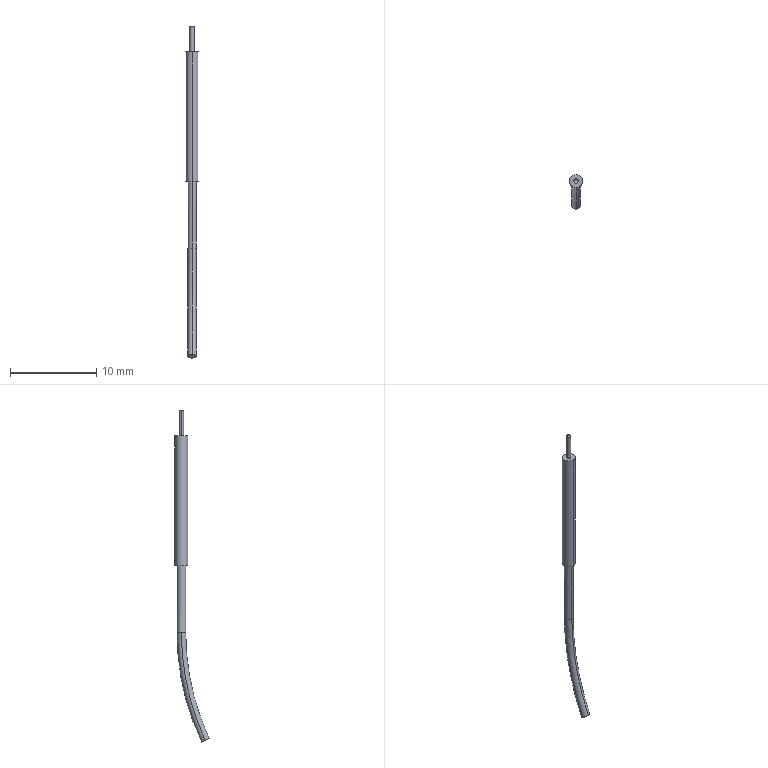Part | NX | 1 solid | 16 faces | box 1.5 x 3.958 x 38.402 mm | volume 43.25 mm3 | cylinder 8 | plane 5 | torus 3 | commonest cylinder face diameters 0.49 x2 0.5 x2 1 x2 1.5 x2
STEP:
#1=CARTESIAN_POINT('',(0.25,0.,3.));
#2=VERTEX_POINT('',#1);
#3=CARTESIAN_POINT('',(-0.25,0.,3.));
#4=VERTEX_POINT('',#3);
#5=CARTESIAN_POINT('',(0.,0.,3.));
#6=DIRECTION('',(0.,0.,-1.));
#7=DIRECTION('',(1.,0.,0.));
#8=AXIS2_PLACEMENT_3D('',#5,#6,#7);
#9=CIRCLE('',#8,0.25);
#10=EDGE_CURVE('',#2,#4,#9,.T.);
#11=ORIENTED_EDGE('',*,*,#10,.F.);
#12=CARTESIAN_POINT('',(0.,0.,3.));
#13=DIRECTION('',(0.,0.,-1.));
#14=DIRECTION('',(1.,0.,0.));
#15=AXIS2_PLACEMENT_3D('',#12,#13,#14);
#16=CIRCLE('',#15,0.25);
#17=EDGE_CURVE('',#4,#2,#16,.T.);
#18=ORIENTED_EDGE('',*,*,#17,.F.);
#19=EDGE_LOOP('',(#11,#18));
#20=FACE_BOUND('',#19,.T.);
#21=CARTESIAN_POINT('',(-0.245,0.,3.));
#22=VERTEX_POINT('',#21);
#23=CARTESIAN_POINT('',(0.245,0.,3.));
#24=VERTEX_POINT('',#23);
#25=CARTESIAN_POINT('',(0.,0.,3.));
#26=DIRECTION('',(0.,0.,1.));
#27=DIRECTION('',(1.,0.,0.));
#28=AXIS2_PLACEMENT_3D('',#25,#26,#27);
#29=CIRCLE('',#28,0.245);
#30=EDGE_CURVE('',#22,#24,#29,.T.);
#31=ORIENTED_EDGE('',*,*,#30,.F.);
#32=CARTESIAN_POINT('',(0.,0.,3.));
#33=DIRECTION('',(0.,0.,1.));
#34=DIRECTION('',(1.,0.,0.));
#35=AXIS2_PLACEMENT_3D('',#32,#33,#34);
#36=CIRCLE('',#35,0.245);
#37=EDGE_CURVE('',#24,#22,#36,.T.);
#38=ORIENTED_EDGE('',*,*,#37,.F.);
#39=EDGE_LOOP('',(#31,#38));
#40=FACE_BOUND('',#39,.T.);
#41=CARTESIAN_POINT('',(0.,0.,3.));
#42=DIRECTION('',(0.,0.,1.));
#43=DIRECTION('',(1.,0.,0.));
#44=AXIS2_PLACEMENT_3D('',#41,#42,#43);
#45=PLANE('',#44);
#46=ADVANCED_FACE('',(#20,#40),#45,.T.);
#47=ORIENTED_EDGE('',*,*,#10,.T.);
#48=CARTESIAN_POINT('',(-0.25,0.,0.));
#49=VERTEX_POINT('',#48);
#50=CARTESIAN_POINT('',(-0.25,0.,0.));
#51=DIRECTION('',(0.,0.,1.));
#52=VECTOR('',#51,1000.);
#53=LINE('',#50,#52);
#54=EDGE_CURVE('',#49,#4,#53,.T.);
#55=ORIENTED_EDGE('',*,*,#54,.F.);
#56=CARTESIAN_POINT('',(0.25,0.,0.));
#57=VERTEX_POINT('',#56);
#58=CARTESIAN_POINT('',(0.,0.,0.));
#59=DIRECTION('',(0.,0.,1.));
#60=DIRECTION('',(-1.,0.,0.));
#61=AXIS2_PLACEMENT_3D('',#58,#59,#60);
#62=CIRCLE('',#61,0.25);
#63=EDGE_CURVE('',#49,#57,#62,.T.);
#64=ORIENTED_EDGE('',*,*,#63,.T.);
#65=CARTESIAN_POINT('',(0.25,0.,0.));
#66=DIRECTION('',(0.,0.,1.));
#67=VECTOR('',#66,1000.);
#68=LINE('',#65,#67);
#69=EDGE_CURVE('',#57,#2,#68,.T.);
#70=ORIENTED_EDGE('',*,*,#69,.T.);
#71=EDGE_LOOP('',(#47,#55,#64,#70));
#72=FACE_BOUND('',#71,.T.);
#73=CARTESIAN_POINT('',(0.,0.,0.));
#74=DIRECTION('',(0.,0.,1.));
#75=DIRECTION('',(1.,0.,0.));
#76=AXIS2_PLACEMENT_3D('',#73,#74,#75);
#77=CYLINDRICAL_SURFACE('',#76,0.25);
#78=ADVANCED_FACE('',(#72),#77,.T.);
#79=CARTESIAN_POINT('',(0.,-0.75,0.));
#80=VERTEX_POINT('',#79);
#81=CARTESIAN_POINT('',(0.,0.75,0.));
#82=VERTEX_POINT('',#81);
#83=CARTESIAN_POINT('',(0.,0.,0.));
#84=DIRECTION('',(0.,0.,-1.));
#85=DIRECTION('',(0.,1.,0.));
#86=AXIS2_PLACEMENT_3D('',#83,#84,#85);
#87=CIRCLE('',#86,0.75);
#88=EDGE_CURVE('',#80,#82,#87,.T.);
#89=ORIENTED_EDGE('',*,*,#88,.F.);
#90=CARTESIAN_POINT('',(0.,0.,0.));
#91=DIRECTION('',(0.,0.,-1.));
#92=DIRECTION('',(0.,1.,0.));
#93=AXIS2_PLACEMENT_3D('',#90,#91,#92);
#94=CIRCLE('',#93,0.75);
#95=EDGE_CURVE('',#82,#80,#94,.T.);
#96=ORIENTED_EDGE('',*,*,#95,.F.);
#97=EDGE_LOOP('',(#89,#96));
#98=FACE_BOUND('',#97,.T.);
#99=ORIENTED_EDGE('',*,*,#63,.F.);
#100=CARTESIAN_POINT('',(0.,0.,0.));
#101=DIRECTION('',(0.,0.,1.));
#102=DIRECTION('',(-1.,0.,0.));
#103=AXIS2_PLACEMENT_3D('',#100,#101,#102);
#104=CIRCLE('',#103,0.25);
#105=EDGE_CURVE('',#57,#49,#104,.T.);
#106=ORIENTED_EDGE('',*,*,#105,.F.);
#107=EDGE_LOOP('',(#99,#106));
#108=FACE_BOUND('',#107,.T.);
#109=CARTESIAN_POINT('',(0.,0.,0.));
#110=DIRECTION('',(0.,0.,-1.));
#111=DIRECTION('',(0.,-1.,0.));
#112=AXIS2_PLACEMENT_3D('',#109,#110,#111);
#113=PLANE('',#112);
#114=ADVANCED_FACE('',(#98,#108),#113,.F.);
#115=CARTESIAN_POINT('',(0.,0.75,-15.));
#116=VERTEX_POINT('',#115);
#117=CARTESIAN_POINT('',(0.,-0.75,-15.));
#118=VERTEX_POINT('',#117);
#119=CARTESIAN_POINT('',(0.,0.,-15.));
#120=DIRECTION('',(0.,0.,1.));
#121=DIRECTION('',(0.,1.,0.));
#122=AXIS2_PLACEMENT_3D('',#119,#120,#121);
#123=CIRCLE('',#122,0.75);
#124=EDGE_CURVE('',#116,#118,#123,.T.);
#125=ORIENTED_EDGE('',*,*,#124,.T.);
#126=CARTESIAN_POINT('',(0.,-0.75,0.));
#127=DIRECTION('',(0.,0.,-1.));
#128=VECTOR('',#127,1000.);
#129=LINE('',#126,#128);
#130=EDGE_CURVE('',#118,#80,#129,.F.);
#131=ORIENTED_EDGE('',*,*,#130,.T.);
#132=ORIENTED_EDGE('',*,*,#88,.T.);
#133=CARTESIAN_POINT('',(0.,0.75,0.));
#134=DIRECTION('',(0.,0.,-1.));
#135=VECTOR('',#134,1000.);
#136=LINE('',#133,#135);
#137=EDGE_CURVE('',#116,#82,#136,.F.);
#138=ORIENTED_EDGE('',*,*,#137,.F.);
#139=EDGE_LOOP('',(#125,#131,#132,#138));
#140=FACE_BOUND('',#139,.T.);
#141=CARTESIAN_POINT('',(0.,0.,0.));
#142=DIRECTION('',(0.,0.,-1.));
#143=DIRECTION('',(0.,-1.,0.));
#144=AXIS2_PLACEMENT_3D('',#141,#142,#143);
#145=CYLINDRICAL_SURFACE('',#144,0.75);
#146=ADVANCED_FACE('',(#140),#145,.T.);
#147=CARTESIAN_POINT('',(-0.5,-2.754,-35.192));
#148=VERTEX_POINT('',#147);
#149=CARTESIAN_POINT('',(0.,-3.208,-34.982));
#150=VERTEX_POINT('',#149);
#151=CARTESIAN_POINT('',(0.,-2.754,-35.192));
#152=DIRECTION('',(0.,0.4199,0.9076));
#153=DIRECTION('',(0.,-0.9076,0.4199));
#154=AXIS2_PLACEMENT_3D('',#151,#152,#153);
#155=CIRCLE('',#154,0.5);
#156=EDGE_CURVE('',#148,#150,#155,.T.);
#157=ORIENTED_EDGE('',*,*,#156,.F.);
#158=CARTESIAN_POINT('',(0.5,-2.754,-35.192));
#159=VERTEX_POINT('',#158);
#160=CARTESIAN_POINT('',(0.,-2.754,-35.192));
#161=DIRECTION('',(0.,0.4199,0.9076));
#162=DIRECTION('',(0.,-0.9076,0.4199));
#163=AXIS2_PLACEMENT_3D('',#160,#161,#162);
#164=CIRCLE('',#163,0.5);
#165=EDGE_CURVE('',#159,#148,#164,.T.);
#166=ORIENTED_EDGE('',*,*,#165,.F.);
#167=CARTESIAN_POINT('',(0.,-2.754,-35.192));
#168=DIRECTION('',(0.,0.4199,0.9076));
#169=DIRECTION('',(0.,-0.9076,0.4199));
#170=AXIS2_PLACEMENT_3D('',#167,#168,#169);
#171=CIRCLE('',#170,0.5);
#172=EDGE_CURVE('',#150,#159,#171,.T.);
#173=ORIENTED_EDGE('',*,*,#172,.F.);
#174=EDGE_LOOP('',(#157,#166,#173));
#175=FACE_BOUND('',#174,.T.);
#176=CARTESIAN_POINT('',(1.,-29.794,-22.681));
#177=DIRECTION('',(0.,-0.4199,-0.9076));
#178=DIRECTION('',(0.,-0.9076,0.4199));
#179=AXIS2_PLACEMENT_3D('',#176,#177,#178);
#180=PLANE('',#179);
#181=ADVANCED_FACE('',(#175),#180,.T.);
#182=ORIENTED_EDGE('',*,*,#124,.F.);
#183=CARTESIAN_POINT('',(0.,0.,-15.));
#184=DIRECTION('',(0.,0.,1.));
#185=DIRECTION('',(0.,1.,0.));
#186=AXIS2_PLACEMENT_3D('',#183,#184,#185);
#187=CIRCLE('',#186,0.75);
#188=EDGE_CURVE('',#118,#116,#187,.T.);
#189=ORIENTED_EDGE('',*,*,#188,.F.);
#190=EDGE_LOOP('',(#182,#189));
#191=FACE_BOUND('',#190,.T.);
#192=CARTESIAN_POINT('',(0.,0.5,-15.));
#193=VERTEX_POINT('',#192);
#194=CARTESIAN_POINT('',(0.,-0.5,-15.));
#195=VERTEX_POINT('',#194);
#196=CARTESIAN_POINT('',(0.,0.,-15.));
#197=DIRECTION('',(0.,0.,-1.));
#198=DIRECTION('',(0.,-1.,0.));
#199=AXIS2_PLACEMENT_3D('',#196,#197,#198);
#200=CIRCLE('',#199,0.5);
#201=EDGE_CURVE('',#193,#195,#200,.T.);
#202=ORIENTED_EDGE('',*,*,#201,.F.);
#203=CARTESIAN_POINT('',(0.,0.,-15.));
#204=DIRECTION('',(0.,0.,-1.));
#205=DIRECTION('',(0.,-1.,0.));
#206=AXIS2_PLACEMENT_3D('',#203,#204,#205);
#207=CIRCLE('',#206,0.5);
#208=EDGE_CURVE('',#195,#193,#207,.T.);
#209=ORIENTED_EDGE('',*,*,#208,.F.);
#210=EDGE_LOOP('',(#202,#209));
#211=FACE_BOUND('',#210,.T.);
#212=CARTESIAN_POINT('',(0.,0.,-15.));
#213=DIRECTION('',(0.,0.,-1.));
#214=DIRECTION('',(0.,-1.,0.));
#215=AXIS2_PLACEMENT_3D('',#212,#213,#214);
#216=PLANE('',#215);
#217=ADVANCED_FACE('',(#191,#211),#216,.T.);
#218=ORIENTED_EDGE('',*,*,#201,.T.);
#219=CARTESIAN_POINT('',(0.,-0.5,-22.681));
#220=VERTEX_POINT('',#219);
#221=CARTESIAN_POINT('',(0.,-0.5,-15.));
#222=DIRECTION('',(0.,0.,-1.));
#223=VECTOR('',#222,1000.);
#224=LINE('',#221,#223);
#225=EDGE_CURVE('',#195,#220,#224,.T.);
#226=ORIENTED_EDGE('',*,*,#225,.T.);
#227=CARTESIAN_POINT('',(0.5,0.,-22.681));
#228=VERTEX_POINT('',#227);
#229=CARTESIAN_POINT('',(0.,0.,-22.681));
#230=DIRECTION('',(0.,0.,-1.));
#231=DIRECTION('',(-1.,0.,0.));
#232=AXIS2_PLACEMENT_3D('',#229,#230,#231);
#233=CIRCLE('',#232,0.5);
#234=EDGE_CURVE('',#228,#220,#233,.T.);
#235=ORIENTED_EDGE('',*,*,#234,.F.);
#236=CARTESIAN_POINT('',(0.,0.5,-22.681));
#237=VERTEX_POINT('',#236);
#238=CARTESIAN_POINT('',(0.,0.,-22.681));
#239=DIRECTION('',(0.,0.,-1.));
#240=DIRECTION('',(-1.,0.,0.));
#241=AXIS2_PLACEMENT_3D('',#238,#239,#240);
#242=CIRCLE('',#241,0.5);
#243=EDGE_CURVE('',#237,#228,#242,.T.);
#244=ORIENTED_EDGE('',*,*,#243,.F.);
#245=CARTESIAN_POINT('',(0.,0.5,-15.));
#246=DIRECTION('',(0.,0.,-1.));
#247=VECTOR('',#246,1000.);
#248=LINE('',#245,#247);
#249=EDGE_CURVE('',#193,#237,#248,.T.);
#250=ORIENTED_EDGE('',*,*,#249,.F.);
#251=EDGE_LOOP('',(#218,#226,#235,#244,#250));
#252=FACE_BOUND('',#251,.T.);
#253=CARTESIAN_POINT('',(0.,0.,-15.));
#254=DIRECTION('',(0.,0.,-1.));
#255=DIRECTION('',(0.,1.,0.));
#256=AXIS2_PLACEMENT_3D('',#253,#254,#255);
#257=CYLINDRICAL_SURFACE('',#256,0.5);
#258=ADVANCED_FACE('',(#252),#257,.T.);
#259=CARTESIAN_POINT('',(-0.245,0.,2.9));
#260=VERTEX_POINT('',#259);
#261=CARTESIAN_POINT('',(0.245,0.,2.9));
#262=VERTEX_POINT('',#261);
#263=CARTESIAN_POINT('',(0.,0.,2.9));
#264=DIRECTION('',(0.,0.,-1.));
#265=DIRECTION('',(-1.,0.,0.));
#266=AXIS2_PLACEMENT_3D('',#263,#264,#265);
#267=CIRCLE('',#266,0.245);
#268=EDGE_CURVE('',#260,#262,#267,.T.);
#269=ORIENTED_EDGE('',*,*,#268,.F.);
#270=CARTESIAN_POINT('',(0.,0.,2.9));
#271=DIRECTION('',(0.,0.,-1.));
#272=DIRECTION('',(-1.,0.,0.));
#273=AXIS2_PLACEMENT_3D('',#270,#271,#272);
#274=CIRCLE('',#273,0.245);
#275=EDGE_CURVE('',#262,#260,#274,.T.);
#276=ORIENTED_EDGE('',*,*,#275,.F.);
#277=EDGE_LOOP('',(#269,#276));
#278=FACE_BOUND('',#277,.T.);
#279=CARTESIAN_POINT('',(0.,0.,2.9));
#280=DIRECTION('',(0.,0.,1.));
#281=DIRECTION('',(1.,0.,0.));
#282=AXIS2_PLACEMENT_3D('',#279,#280,#281);
#283=PLANE('',#282);
#284=ADVANCED_FACE('',(#278),#283,.T.);
#285=CARTESIAN_POINT('',(0.,-29.794,-22.681));
#286=DIRECTION('',(-1.,0.,0.));
#287=DIRECTION('',(0.,0.,1.));
#288=AXIS2_PLACEMENT_3D('',#285,#286,#287);
#289=CIRCLE('',#288,29.294);
#290=EDGE_CURVE('',#220,#150,#289,.T.);
#291=ORIENTED_EDGE('',*,*,#290,.F.);
#292=CARTESIAN_POINT('',(-0.5,0.,-22.681));
#293=VERTEX_POINT('',#292);
#294=CARTESIAN_POINT('',(0.,0.,-22.681));
#295=DIRECTION('',(0.,0.,-1.));
#296=DIRECTION('',(-1.,0.,0.));
#297=AXIS2_PLACEMENT_3D('',#294,#295,#296);
#298=CIRCLE('',#297,0.5);
#299=EDGE_CURVE('',#220,#293,#298,.T.);
#300=ORIENTED_EDGE('',*,*,#299,.T.);
#301=CARTESIAN_POINT('',(-0.5,-29.794,-22.681));
#302=DIRECTION('',(-1.,0.,0.));
#303=DIRECTION('',(0.,1.,0.));
#304=AXIS2_PLACEMENT_3D('',#301,#302,#303);
#305=CIRCLE('',#304,29.794);
#306=EDGE_CURVE('',#293,#148,#305,.T.);
#307=ORIENTED_EDGE('',*,*,#306,.T.);
#308=ORIENTED_EDGE('',*,*,#156,.T.);
#309=EDGE_LOOP('',(#291,#300,#307,#308));
#310=FACE_BOUND('',#309,.T.);
#311=CARTESIAN_POINT('',(0.,-29.794,-22.681));
#312=DIRECTION('',(-1.,0.,0.));
#313=DIRECTION('',(0.,1.,0.));
#314=AXIS2_PLACEMENT_3D('',#311,#312,#313);
#315=TOROIDAL_SURFACE('',#314,29.794,0.5);
#316=ADVANCED_FACE('',(#310),#315,.T.);
#317=ORIENTED_EDGE('',*,*,#30,.T.);
#318=CARTESIAN_POINT('',(0.245,0.,3.));
#319=DIRECTION('',(0.,0.,1.));
#320=VECTOR('',#319,1000.);
#321=LINE('',#318,#320);
#322=EDGE_CURVE('',#262,#24,#321,.T.);
#323=ORIENTED_EDGE('',*,*,#322,.F.);
#324=ORIENTED_EDGE('',*,*,#275,.T.);
#325=CARTESIAN_POINT('',(-0.245,0.,3.));
#326=DIRECTION('',(0.,0.,1.));
#327=VECTOR('',#326,1000.);
#328=LINE('',#325,#327);
#329=EDGE_CURVE('',#260,#22,#328,.T.);
#330=ORIENTED_EDGE('',*,*,#329,.T.);
#331=EDGE_LOOP('',(#317,#323,#324,#330));
#332=FACE_BOUND('',#331,.T.);
#333=CARTESIAN_POINT('',(0.,0.,3.));
#334=DIRECTION('',(0.,0.,1.));
#335=DIRECTION('',(-1.,0.,0.));
#336=AXIS2_PLACEMENT_3D('',#333,#334,#335);
#337=CYLINDRICAL_SURFACE('',#336,0.245);
#338=ADVANCED_FACE('',(#332),#337,.F.);
#339=ORIENTED_EDGE('',*,*,#306,.F.);
#340=CARTESIAN_POINT('',(0.,0.,-22.681));
#341=DIRECTION('',(0.,0.,-1.));
#342=DIRECTION('',(-1.,0.,0.));
#343=AXIS2_PLACEMENT_3D('',#340,#341,#342);
#344=CIRCLE('',#343,0.5);
#345=EDGE_CURVE('',#293,#237,#344,.T.);
#346=ORIENTED_EDGE('',*,*,#345,.T.);
#347=ORIENTED_EDGE('',*,*,#243,.T.);
#348=CARTESIAN_POINT('',(0.5,-29.794,-22.681));
#349=DIRECTION('',(-1.,0.,0.));
#350=DIRECTION('',(0.,1.,0.));
#351=AXIS2_PLACEMENT_3D('',#348,#349,#350);
#352=CIRCLE('',#351,29.794);
#353=EDGE_CURVE('',#228,#159,#352,.T.);
#354=ORIENTED_EDGE('',*,*,#353,.T.);
#355=ORIENTED_EDGE('',*,*,#165,.T.);
#356=EDGE_LOOP('',(#339,#346,#347,#354,#355));
#357=FACE_BOUND('',#356,.T.);
#358=CARTESIAN_POINT('',(0.,-29.794,-22.681));
#359=DIRECTION('',(-1.,0.,0.));
#360=DIRECTION('',(0.,1.,0.));
#361=AXIS2_PLACEMENT_3D('',#358,#359,#360);
#362=TOROIDAL_SURFACE('',#361,29.794,0.5);
#363=ADVANCED_FACE('',(#357),#362,.T.);
#364=ORIENTED_EDGE('',*,*,#130,.F.);
#365=ORIENTED_EDGE('',*,*,#188,.T.);
#366=ORIENTED_EDGE('',*,*,#137,.T.);
#367=ORIENTED_EDGE('',*,*,#95,.T.);
#368=EDGE_LOOP('',(#364,#365,#366,#367));
#369=FACE_BOUND('',#368,.T.);
#370=CARTESIAN_POINT('',(0.,0.,0.));
#371=DIRECTION('',(0.,0.,-1.));
#372=DIRECTION('',(0.,-1.,0.));
#373=AXIS2_PLACEMENT_3D('',#370,#371,#372);
#374=CYLINDRICAL_SURFACE('',#373,0.75);
#375=ADVANCED_FACE('',(#369),#374,.T.);
#376=ORIENTED_EDGE('',*,*,#69,.F.);
#377=ORIENTED_EDGE('',*,*,#105,.T.);
#378=ORIENTED_EDGE('',*,*,#54,.T.);
#379=ORIENTED_EDGE('',*,*,#17,.T.);
#380=EDGE_LOOP('',(#376,#377,#378,#379));
#381=FACE_BOUND('',#380,.T.);
#382=CARTESIAN_POINT('',(0.,0.,0.));
#383=DIRECTION('',(0.,0.,1.));
#384=DIRECTION('',(1.,0.,0.));
#385=AXIS2_PLACEMENT_3D('',#382,#383,#384);
#386=CYLINDRICAL_SURFACE('',#385,0.25);
#387=ADVANCED_FACE('',(#381),#386,.T.);
#388=ORIENTED_EDGE('',*,*,#268,.T.);
#389=ORIENTED_EDGE('',*,*,#322,.T.);
#390=ORIENTED_EDGE('',*,*,#37,.T.);
#391=ORIENTED_EDGE('',*,*,#329,.F.);
#392=EDGE_LOOP('',(#388,#389,#390,#391));
#393=FACE_BOUND('',#392,.T.);
#394=CARTESIAN_POINT('',(0.,0.,3.));
#395=DIRECTION('',(0.,0.,1.));
#396=DIRECTION('',(-1.,0.,0.));
#397=AXIS2_PLACEMENT_3D('',#394,#395,#396);
#398=CYLINDRICAL_SURFACE('',#397,0.245);
#399=ADVANCED_FACE('',(#393),#398,.F.);
#400=ORIENTED_EDGE('',*,*,#249,.T.);
#401=ORIENTED_EDGE('',*,*,#345,.F.);
#402=ORIENTED_EDGE('',*,*,#299,.F.);
#403=ORIENTED_EDGE('',*,*,#225,.F.);
#404=ORIENTED_EDGE('',*,*,#208,.T.);
#405=EDGE_LOOP('',(#400,#401,#402,#403,#404));
#406=FACE_BOUND('',#405,.T.);
#407=CARTESIAN_POINT('',(0.,0.,-15.));
#408=DIRECTION('',(0.,0.,-1.));
#409=DIRECTION('',(0.,1.,0.));
#410=AXIS2_PLACEMENT_3D('',#407,#408,#409);
#411=CYLINDRICAL_SURFACE('',#410,0.5);
#412=ADVANCED_FACE('',(#406),#411,.T.);
#413=ORIENTED_EDGE('',*,*,#234,.T.);
#414=ORIENTED_EDGE('',*,*,#290,.T.);
#415=ORIENTED_EDGE('',*,*,#172,.T.);
#416=ORIENTED_EDGE('',*,*,#353,.F.);
#417=EDGE_LOOP('',(#413,#414,#415,#416));
#418=FACE_BOUND('',#417,.T.);
#419=CARTESIAN_POINT('',(0.,-29.794,-22.681));
#420=DIRECTION('',(-1.,0.,0.));
#421=DIRECTION('',(0.,1.,0.));
#422=AXIS2_PLACEMENT_3D('',#419,#420,#421);
#423=TOROIDAL_SURFACE('',#422,29.794,0.5);
#424=ADVANCED_FACE('',(#418),#423,.T.);
#425=CLOSED_SHELL('',(#46,#78,#114,#146,#181,#217,#258,#284,#316,#338,#363,#375,#387,#399,#412,#424));
#426=MANIFOLD_SOLID_BREP('',#425);
#427=(LENGTH_UNIT()NAMED_UNIT(*)SI_UNIT(.MILLI.,.METRE.));
#428=UNCERTAINTY_MEASURE_WITH_UNIT(LENGTH_MEASURE(0.00001),#427,'','');
#429=(NAMED_UNIT(*)PLANE_ANGLE_UNIT()SI_UNIT($,.RADIAN.));
#430=(NAMED_UNIT(*)SI_UNIT($,.STERADIAN.)SOLID_ANGLE_UNIT());
#431=(GEOMETRIC_REPRESENTATION_CONTEXT(3)GLOBAL_UNCERTAINTY_ASSIGNED_CONTEXT((#428))GLOBAL_UNIT_ASSIGNED_CONTEXT((#427,#429,#430))REPRESENTATION_CONTEXT('',''));
#432=ADVANCED_BREP_SHAPE_REPRESENTATION('',(#426),#431);